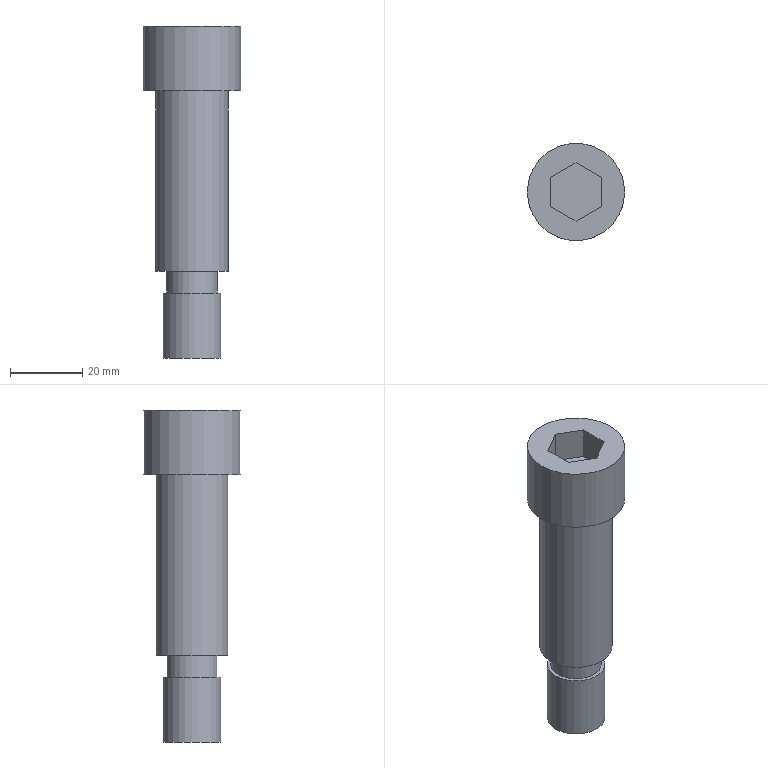Part | NX | features solid 2 | 1 solid | 16 faces | box 27 x 27 x 92 mm | volume 29029 mm3 | plane 12 | cylinder 4 | commonest cylinder face diameters 14 x1 16 x1 20 x1 27 x1
STEP:
#1=CARTESIAN_POINT('',(727.081,-220.938,-70.));
#2=VERTEX_POINT('',#1);
#3=CARTESIAN_POINT('',(717.081,-220.938,-70.));
#4=DIRECTION('',(0.,0.,1.));
#5=DIRECTION('',(1.,0.,0.));
#6=AXIS2_PLACEMENT_3D('',#3,#4,#5);
#7=CIRCLE('',#6,10.);
#8=EDGE_CURVE('',#2,#2,#7,.T.);
#9=ORIENTED_EDGE('',*,*,#8,.T.);
#10=EDGE_LOOP('',(#9));
#11=FACE_BOUND('',#10,.T.);
#12=CARTESIAN_POINT('',(707.081,-220.938,-20.));
#13=VERTEX_POINT('',#12);
#14=CARTESIAN_POINT('',(717.081,-220.938,-20.));
#15=DIRECTION('',(0.,0.,-1.));
#16=DIRECTION('',(-1.,0.,0.));
#17=AXIS2_PLACEMENT_3D('',#14,#15,#16);
#18=CIRCLE('',#17,10.);
#19=EDGE_CURVE('',#13,#13,#18,.T.);
#20=ORIENTED_EDGE('',*,*,#19,.T.);
#21=EDGE_LOOP('',(#20));
#22=FACE_BOUND('',#21,.T.);
#23=CARTESIAN_POINT('',(717.081,-220.938,-20.));
#24=DIRECTION('',(0.,0.,-1.));
#25=DIRECTION('',(1.,0.,0.));
#26=AXIS2_PLACEMENT_3D('',#23,#24,#25);
#27=CYLINDRICAL_SURFACE('',#26,10.);
#28=ADVANCED_FACE('',(#11,#22),#27,.T.);
#29=CARTESIAN_POINT('',(703.581,-220.938,-2.));
#30=VERTEX_POINT('',#29);
#31=CARTESIAN_POINT('',(717.081,-220.938,-2.));
#32=DIRECTION('',(0.,0.,-1.));
#33=DIRECTION('',(-1.,0.,0.));
#34=AXIS2_PLACEMENT_3D('',#31,#32,#33);
#35=CIRCLE('',#34,13.5);
#36=EDGE_CURVE('',#30,#30,#35,.T.);
#37=ORIENTED_EDGE('',*,*,#36,.F.);
#38=EDGE_LOOP('',(#37));
#39=FACE_BOUND('',#38,.T.);
#40=CARTESIAN_POINT('',(724.081,-224.98,-2.));
#41=VERTEX_POINT('',#40);
#42=CARTESIAN_POINT('',(724.081,-216.896,-2.));
#43=VERTEX_POINT('',#42);
#44=CARTESIAN_POINT('',(724.081,-220.938,-2.));
#45=DIRECTION('',(0.,1.,0.));
#46=VECTOR('',#45,1000.);
#47=LINE('',#44,#46);
#48=EDGE_CURVE('',#41,#43,#47,.T.);
#49=ORIENTED_EDGE('',*,*,#48,.F.);
#50=CARTESIAN_POINT('',(717.081,-229.021,-2.));
#51=VERTEX_POINT('',#50);
#52=CARTESIAN_POINT('',(720.581,-227.,-2.));
#53=DIRECTION('',(0.866,0.5,0.));
#54=VECTOR('',#53,1000.);
#55=LINE('',#52,#54);
#56=EDGE_CURVE('',#51,#41,#55,.T.);
#57=ORIENTED_EDGE('',*,*,#56,.F.);
#58=CARTESIAN_POINT('',(710.081,-224.98,-2.));
#59=VERTEX_POINT('',#58);
#60=CARTESIAN_POINT('',(713.581,-227.,-2.));
#61=DIRECTION('',(0.866,-0.5,0.));
#62=VECTOR('',#61,1000.);
#63=LINE('',#60,#62);
#64=EDGE_CURVE('',#59,#51,#63,.T.);
#65=ORIENTED_EDGE('',*,*,#64,.F.);
#66=CARTESIAN_POINT('',(710.081,-216.896,-2.));
#67=VERTEX_POINT('',#66);
#68=CARTESIAN_POINT('',(710.081,-220.938,-2.));
#69=DIRECTION('',(0.,-1.,0.));
#70=VECTOR('',#69,1000.);
#71=LINE('',#68,#70);
#72=EDGE_CURVE('',#67,#59,#71,.T.);
#73=ORIENTED_EDGE('',*,*,#72,.F.);
#74=CARTESIAN_POINT('',(717.081,-212.855,-2.));
#75=VERTEX_POINT('',#74);
#76=CARTESIAN_POINT('',(713.581,-214.876,-2.));
#77=DIRECTION('',(-0.866,-0.5,0.));
#78=VECTOR('',#77,1000.);
#79=LINE('',#76,#78);
#80=EDGE_CURVE('',#75,#67,#79,.T.);
#81=ORIENTED_EDGE('',*,*,#80,.F.);
#82=CARTESIAN_POINT('',(720.581,-214.876,-2.));
#83=DIRECTION('',(-0.866,0.5,0.));
#84=VECTOR('',#83,1000.);
#85=LINE('',#82,#84);
#86=EDGE_CURVE('',#43,#75,#85,.T.);
#87=ORIENTED_EDGE('',*,*,#86,.F.);
#88=EDGE_LOOP('',(#49,#57,#65,#73,#81,#87));
#89=FACE_BOUND('',#88,.T.);
#90=CARTESIAN_POINT('',(717.081,-220.938,-2.));
#91=DIRECTION('',(0.,0.,1.));
#92=DIRECTION('',(-1.,0.,0.));
#93=AXIS2_PLACEMENT_3D('',#90,#91,#92);
#94=PLANE('',#93);
#95=ADVANCED_FACE('',(#39,#89),#94,.T.);
#96=CARTESIAN_POINT('',(703.581,-220.938,-20.));
#97=VERTEX_POINT('',#96);
#98=CARTESIAN_POINT('',(717.081,-220.938,-20.));
#99=DIRECTION('',(0.,0.,-1.));
#100=DIRECTION('',(-1.,0.,0.));
#101=AXIS2_PLACEMENT_3D('',#98,#99,#100);
#102=CIRCLE('',#101,13.5);
#103=EDGE_CURVE('',#97,#97,#102,.T.);
#104=ORIENTED_EDGE('',*,*,#103,.T.);
#105=EDGE_LOOP('',(#104));
#106=FACE_BOUND('',#105,.T.);
#107=ORIENTED_EDGE('',*,*,#19,.F.);
#108=EDGE_LOOP('',(#107));
#109=FACE_BOUND('',#108,.T.);
#110=CARTESIAN_POINT('',(717.081,-220.938,-20.));
#111=DIRECTION('',(0.,0.,1.));
#112=DIRECTION('',(-1.,0.,0.));
#113=AXIS2_PLACEMENT_3D('',#110,#111,#112);
#114=PLANE('',#113);
#115=ADVANCED_FACE('',(#106,#109),#114,.F.);
#116=ORIENTED_EDGE('',*,*,#36,.T.);
#117=EDGE_LOOP('',(#116));
#118=FACE_BOUND('',#117,.T.);
#119=ORIENTED_EDGE('',*,*,#103,.F.);
#120=EDGE_LOOP('',(#119));
#121=FACE_BOUND('',#120,.T.);
#122=CARTESIAN_POINT('',(717.081,-220.938,-2.));
#123=DIRECTION('',(0.,0.,-1.));
#124=DIRECTION('',(1.,0.,0.));
#125=AXIS2_PLACEMENT_3D('',#122,#123,#124);
#126=CYLINDRICAL_SURFACE('',#125,13.5);
#127=ADVANCED_FACE('',(#118,#121),#126,.T.);
#128=CARTESIAN_POINT('',(724.081,-216.896,-11.));
#129=VERTEX_POINT('',#128);
#130=CARTESIAN_POINT('',(724.081,-216.896,9.));
#131=DIRECTION('',(0.,0.,-1.));
#132=VECTOR('',#131,1000.);
#133=LINE('',#130,#132);
#134=EDGE_CURVE('',#43,#129,#133,.T.);
#135=ORIENTED_EDGE('',*,*,#134,.F.);
#136=ORIENTED_EDGE('',*,*,#86,.T.);
#137=CARTESIAN_POINT('',(717.081,-212.855,-11.));
#138=VERTEX_POINT('',#137);
#139=CARTESIAN_POINT('',(717.081,-212.855,9.));
#140=DIRECTION('',(0.,0.,-1.));
#141=VECTOR('',#140,1000.);
#142=LINE('',#139,#141);
#143=EDGE_CURVE('',#75,#138,#142,.T.);
#144=ORIENTED_EDGE('',*,*,#143,.T.);
#145=CARTESIAN_POINT('',(717.081,-212.855,-11.));
#146=DIRECTION('',(0.866,-0.5,0.));
#147=VECTOR('',#146,1000.);
#148=LINE('',#145,#147);
#149=EDGE_CURVE('',#138,#129,#148,.T.);
#150=ORIENTED_EDGE('',*,*,#149,.T.);
#151=EDGE_LOOP('',(#135,#136,#144,#150));
#152=FACE_BOUND('',#151,.T.);
#153=CARTESIAN_POINT('',(717.081,-212.855,9.));
#154=DIRECTION('',(-0.5,-0.866,0.));
#155=DIRECTION('',(-0.866,0.5,0.));
#156=AXIS2_PLACEMENT_3D('',#153,#154,#155);
#157=PLANE('',#156);
#158=ADVANCED_FACE('',(#152),#157,.T.);
#159=CARTESIAN_POINT('',(724.081,-224.98,-11.));
#160=VERTEX_POINT('',#159);
#161=CARTESIAN_POINT('',(724.081,-224.98,9.));
#162=DIRECTION('',(0.,0.,-1.));
#163=VECTOR('',#162,1000.);
#164=LINE('',#161,#163);
#165=EDGE_CURVE('',#41,#160,#164,.T.);
#166=ORIENTED_EDGE('',*,*,#165,.F.);
#167=ORIENTED_EDGE('',*,*,#48,.T.);
#168=ORIENTED_EDGE('',*,*,#134,.T.);
#169=CARTESIAN_POINT('',(724.081,-216.896,-11.));
#170=DIRECTION('',(0.,-1.,0.));
#171=VECTOR('',#170,1000.);
#172=LINE('',#169,#171);
#173=EDGE_CURVE('',#129,#160,#172,.T.);
#174=ORIENTED_EDGE('',*,*,#173,.T.);
#175=EDGE_LOOP('',(#166,#167,#168,#174));
#176=FACE_BOUND('',#175,.T.);
#177=CARTESIAN_POINT('',(724.081,-216.896,9.));
#178=DIRECTION('',(-1.,0.,0.));
#179=DIRECTION('',(0.,0.,-1.));
#180=AXIS2_PLACEMENT_3D('',#177,#178,#179);
#181=PLANE('',#180);
#182=ADVANCED_FACE('',(#176),#181,.T.);
#183=CARTESIAN_POINT('',(717.081,-229.021,-11.));
#184=VERTEX_POINT('',#183);
#185=CARTESIAN_POINT('',(717.081,-229.021,9.));
#186=DIRECTION('',(0.,0.,-1.));
#187=VECTOR('',#186,1000.);
#188=LINE('',#185,#187);
#189=EDGE_CURVE('',#51,#184,#188,.T.);
#190=ORIENTED_EDGE('',*,*,#189,.F.);
#191=ORIENTED_EDGE('',*,*,#56,.T.);
#192=ORIENTED_EDGE('',*,*,#165,.T.);
#193=CARTESIAN_POINT('',(724.081,-224.98,-11.));
#194=DIRECTION('',(-0.866,-0.5,0.));
#195=VECTOR('',#194,1000.);
#196=LINE('',#193,#195);
#197=EDGE_CURVE('',#160,#184,#196,.T.);
#198=ORIENTED_EDGE('',*,*,#197,.T.);
#199=EDGE_LOOP('',(#190,#191,#192,#198));
#200=FACE_BOUND('',#199,.T.);
#201=CARTESIAN_POINT('',(724.081,-224.98,9.));
#202=DIRECTION('',(-0.5,0.866,0.));
#203=DIRECTION('',(0.866,0.5,0.));
#204=AXIS2_PLACEMENT_3D('',#201,#202,#203);
#205=PLANE('',#204);
#206=ADVANCED_FACE('',(#200),#205,.T.);
#207=CARTESIAN_POINT('',(710.081,-224.98,-11.));
#208=VERTEX_POINT('',#207);
#209=CARTESIAN_POINT('',(710.081,-224.98,9.));
#210=DIRECTION('',(0.,0.,-1.));
#211=VECTOR('',#210,1000.);
#212=LINE('',#209,#211);
#213=EDGE_CURVE('',#59,#208,#212,.T.);
#214=ORIENTED_EDGE('',*,*,#213,.F.);
#215=ORIENTED_EDGE('',*,*,#64,.T.);
#216=ORIENTED_EDGE('',*,*,#189,.T.);
#217=CARTESIAN_POINT('',(717.081,-229.021,-11.));
#218=DIRECTION('',(-0.866,0.5,0.));
#219=VECTOR('',#218,1000.);
#220=LINE('',#217,#219);
#221=EDGE_CURVE('',#184,#208,#220,.T.);
#222=ORIENTED_EDGE('',*,*,#221,.T.);
#223=EDGE_LOOP('',(#214,#215,#216,#222));
#224=FACE_BOUND('',#223,.T.);
#225=CARTESIAN_POINT('',(717.081,-229.021,9.));
#226=DIRECTION('',(0.5,0.866,0.));
#227=DIRECTION('',(0.866,-0.5,0.));
#228=AXIS2_PLACEMENT_3D('',#225,#226,#227);
#229=PLANE('',#228);
#230=ADVANCED_FACE('',(#224),#229,.T.);
#231=CARTESIAN_POINT('',(710.081,-216.896,-11.));
#232=VERTEX_POINT('',#231);
#233=CARTESIAN_POINT('',(710.081,-216.896,9.));
#234=DIRECTION('',(0.,0.,-1.));
#235=VECTOR('',#234,1000.);
#236=LINE('',#233,#235);
#237=EDGE_CURVE('',#67,#232,#236,.T.);
#238=ORIENTED_EDGE('',*,*,#237,.F.);
#239=ORIENTED_EDGE('',*,*,#72,.T.);
#240=ORIENTED_EDGE('',*,*,#213,.T.);
#241=CARTESIAN_POINT('',(710.081,-224.98,-11.));
#242=DIRECTION('',(0.,1.,0.));
#243=VECTOR('',#242,1000.);
#244=LINE('',#241,#243);
#245=EDGE_CURVE('',#208,#232,#244,.T.);
#246=ORIENTED_EDGE('',*,*,#245,.T.);
#247=EDGE_LOOP('',(#238,#239,#240,#246));
#248=FACE_BOUND('',#247,.T.);
#249=CARTESIAN_POINT('',(710.081,-224.98,9.));
#250=DIRECTION('',(1.,0.,0.));
#251=DIRECTION('',(0.,0.,1.));
#252=AXIS2_PLACEMENT_3D('',#249,#250,#251);
#253=PLANE('',#252);
#254=ADVANCED_FACE('',(#248),#253,.T.);
#255=ORIENTED_EDGE('',*,*,#143,.F.);
#256=ORIENTED_EDGE('',*,*,#80,.T.);
#257=ORIENTED_EDGE('',*,*,#237,.T.);
#258=CARTESIAN_POINT('',(710.081,-216.896,-11.));
#259=DIRECTION('',(0.866,0.5,0.));
#260=VECTOR('',#259,1000.);
#261=LINE('',#258,#260);
#262=EDGE_CURVE('',#232,#138,#261,.T.);
#263=ORIENTED_EDGE('',*,*,#262,.T.);
#264=EDGE_LOOP('',(#255,#256,#257,#263));
#265=FACE_BOUND('',#264,.T.);
#266=CARTESIAN_POINT('',(710.081,-216.896,9.));
#267=DIRECTION('',(0.5,-0.866,0.));
#268=DIRECTION('',(-0.866,-0.5,0.));
#269=AXIS2_PLACEMENT_3D('',#266,#267,#268);
#270=PLANE('',#269);
#271=ADVANCED_FACE('',(#265),#270,.T.);
#272=ORIENTED_EDGE('',*,*,#149,.F.);
#273=ORIENTED_EDGE('',*,*,#262,.F.);
#274=ORIENTED_EDGE('',*,*,#245,.F.);
#275=ORIENTED_EDGE('',*,*,#221,.F.);
#276=ORIENTED_EDGE('',*,*,#197,.F.);
#277=ORIENTED_EDGE('',*,*,#173,.F.);
#278=EDGE_LOOP('',(#272,#273,#274,#275,#276,#277));
#279=FACE_BOUND('',#278,.T.);
#280=CARTESIAN_POINT('',(731.081,-220.938,-11.));
#281=DIRECTION('',(0.,0.,1.));
#282=DIRECTION('',(-1.,0.,0.));
#283=AXIS2_PLACEMENT_3D('',#280,#281,#282);
#284=PLANE('',#283);
#285=ADVANCED_FACE('',(#279),#284,.T.);
#286=CARTESIAN_POINT('',(724.081,-220.938,-70.));
#287=VERTEX_POINT('',#286);
#288=CARTESIAN_POINT('',(717.081,-220.938,-70.));
#289=DIRECTION('',(0.,0.,1.));
#290=DIRECTION('',(1.,0.,0.));
#291=AXIS2_PLACEMENT_3D('',#288,#289,#290);
#292=CIRCLE('',#291,7.);
#293=EDGE_CURVE('',#287,#287,#292,.T.);
#294=ORIENTED_EDGE('',*,*,#293,.T.);
#295=EDGE_LOOP('',(#294));
#296=FACE_BOUND('',#295,.T.);
#297=ORIENTED_EDGE('',*,*,#8,.F.);
#298=EDGE_LOOP('',(#297));
#299=FACE_BOUND('',#298,.T.);
#300=CARTESIAN_POINT('',(734.042,-194.768,-70.));
#301=DIRECTION('',(0.,0.,-1.));
#302=DIRECTION('',(1.,0.,0.));
#303=AXIS2_PLACEMENT_3D('',#300,#301,#302);
#304=PLANE('',#303);
#305=ADVANCED_FACE('',(#296,#299),#304,.T.);
#306=CARTESIAN_POINT('',(709.081,-220.938,-94.));
#307=VERTEX_POINT('',#306);
#308=CARTESIAN_POINT('',(717.081,-220.938,-94.));
#309=DIRECTION('',(0.,0.,-1.));
#310=DIRECTION('',(-1.,0.,0.));
#311=AXIS2_PLACEMENT_3D('',#308,#309,#310);
#312=CIRCLE('',#311,8.);
#313=EDGE_CURVE('',#307,#307,#312,.T.);
#314=ORIENTED_EDGE('',*,*,#313,.T.);
#315=EDGE_LOOP('',(#314));
#316=FACE_BOUND('',#315,.T.);
#317=CARTESIAN_POINT('',(717.081,-220.938,-94.));
#318=DIRECTION('',(0.,0.,1.));
#319=DIRECTION('',(-1.,0.,0.));
#320=AXIS2_PLACEMENT_3D('',#317,#318,#319);
#321=PLANE('',#320);
#322=ADVANCED_FACE('',(#316),#321,.F.);
#323=ORIENTED_EDGE('',*,*,#313,.F.);
#324=EDGE_LOOP('',(#323));
#325=FACE_BOUND('',#324,.T.);
#326=CARTESIAN_POINT('',(709.081,-220.938,-76.));
#327=VERTEX_POINT('',#326);
#328=CARTESIAN_POINT('',(717.081,-220.938,-76.));
#329=DIRECTION('',(0.,0.,-1.));
#330=DIRECTION('',(-1.,0.,0.));
#331=AXIS2_PLACEMENT_3D('',#328,#329,#330);
#332=CIRCLE('',#331,8.);
#333=EDGE_CURVE('',#327,#327,#332,.T.);
#334=ORIENTED_EDGE('',*,*,#333,.T.);
#335=EDGE_LOOP('',(#334));
#336=FACE_BOUND('',#335,.T.);
#337=CARTESIAN_POINT('',(717.081,-220.938,-94.));
#338=DIRECTION('',(0.,0.,1.));
#339=DIRECTION('',(-1.,0.,0.));
#340=AXIS2_PLACEMENT_3D('',#337,#338,#339);
#341=CYLINDRICAL_SURFACE('',#340,8.);
#342=ADVANCED_FACE('',(#325,#336),#341,.T.);
#343=CARTESIAN_POINT('',(710.081,-220.938,-76.));
#344=VERTEX_POINT('',#343);
#345=CARTESIAN_POINT('',(717.081,-220.938,-76.));
#346=DIRECTION('',(0.,0.,-1.));
#347=DIRECTION('',(-1.,0.,0.));
#348=AXIS2_PLACEMENT_3D('',#345,#346,#347);
#349=CIRCLE('',#348,7.);
#350=EDGE_CURVE('',#344,#344,#349,.F.);
#351=ORIENTED_EDGE('',*,*,#350,.F.);
#352=EDGE_LOOP('',(#351));
#353=FACE_BOUND('',#352,.T.);
#354=ORIENTED_EDGE('',*,*,#333,.F.);
#355=EDGE_LOOP('',(#354));
#356=FACE_BOUND('',#355,.T.);
#357=CARTESIAN_POINT('',(717.081,-220.938,-76.));
#358=DIRECTION('',(0.,0.,1.));
#359=DIRECTION('',(-1.,0.,0.));
#360=AXIS2_PLACEMENT_3D('',#357,#358,#359);
#361=PLANE('',#360);
#362=ADVANCED_FACE('',(#353,#356),#361,.T.);
#363=ORIENTED_EDGE('',*,*,#350,.T.);
#364=EDGE_LOOP('',(#363));
#365=FACE_BOUND('',#364,.T.);
#366=ORIENTED_EDGE('',*,*,#293,.F.);
#367=EDGE_LOOP('',(#366));
#368=FACE_BOUND('',#367,.T.);
#369=CARTESIAN_POINT('',(717.081,-220.938,-76.));
#370=DIRECTION('',(0.,0.,1.));
#371=DIRECTION('',(-1.,0.,0.));
#372=AXIS2_PLACEMENT_3D('',#369,#370,#371);
#373=CYLINDRICAL_SURFACE('',#372,7.);
#374=ADVANCED_FACE('',(#365,#368),#373,.T.);
#375=CLOSED_SHELL('',(#28,#95,#115,#127,#158,#182,#206,#230,#254,#271,#285,#305,#322,#342,#362,#374));
#376=MANIFOLD_SOLID_BREP('',#375);
#377=(LENGTH_UNIT()NAMED_UNIT(*)SI_UNIT(.MILLI.,.METRE.));
#378=UNCERTAINTY_MEASURE_WITH_UNIT(LENGTH_MEASURE(0.00001),#377,'','');
#379=(NAMED_UNIT(*)PLANE_ANGLE_UNIT()SI_UNIT($,.RADIAN.));
#380=(NAMED_UNIT(*)SI_UNIT($,.STERADIAN.)SOLID_ANGLE_UNIT());
#381=(GEOMETRIC_REPRESENTATION_CONTEXT(3)GLOBAL_UNCERTAINTY_ASSIGNED_CONTEXT((#378))GLOBAL_UNIT_ASSIGNED_CONTEXT((#377,#379,#380))REPRESENTATION_CONTEXT('',''));
#382=ADVANCED_BREP_SHAPE_REPRESENTATION('',(#376),#381);